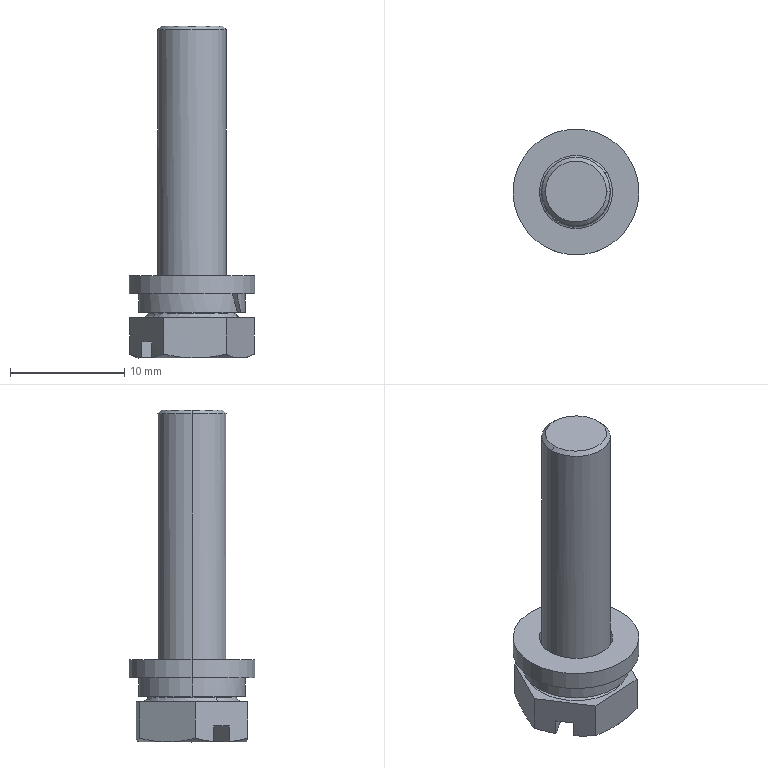Part | SolidWorks | features BaseBody 1 | 1 solid | 46 faces | box 11 x 11 x 29.006 mm | volume 1133 mm3 | plane 19 | cylinder 12 | cone 8 | spline 7 | commonest cylinder face diameters 6.5 x3 9.3 x3 6 x2 6.4 x2 11 x2